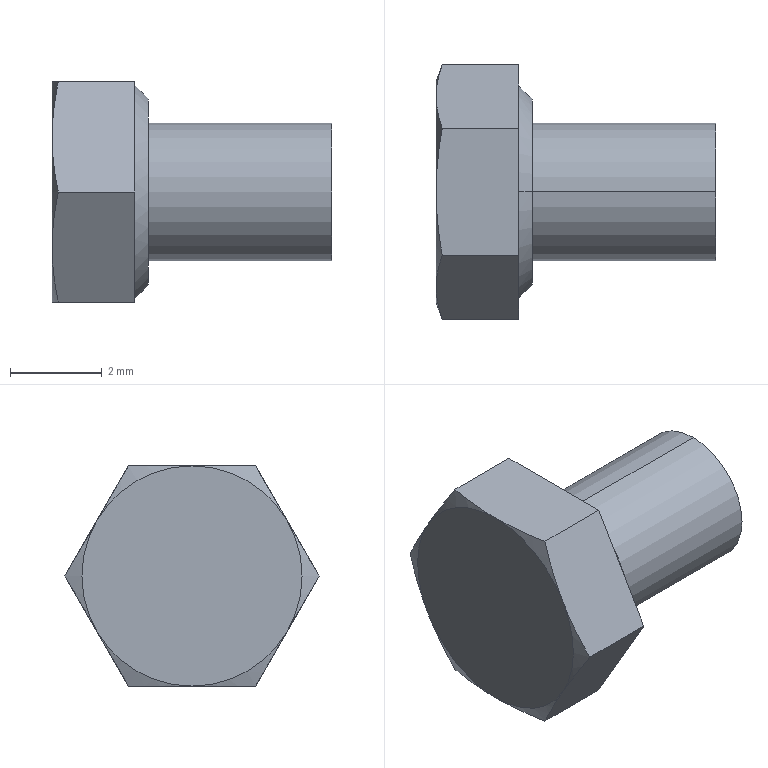Part | SolidWorks | features RevCut 3, Boss 1, Chamfer 1, Extrusion 1, Fillet 1, ICE 1, LPattern 1, Scale 1 | 1 solid | 20 faces | box 6.1 x 5.543 x 4.8 mm | volume 68.566 mm3 | plane 10 | cone 8 | cylinder 2 | commonest cylinder face diameters 3 x2
STEP:
#1=CARTESIAN_POINT('',(4.17,-0.000000444,2.022));
#2=VERTEX_POINT('',#1);
#3=CARTESIAN_POINT('',(4.17,-0.000000444,-2.022));
#4=VERTEX_POINT('',#3);
#5=CARTESIAN_POINT('',(4.17,-0.000000444,0.));
#6=DIRECTION('',(-1.,0.,0.));
#7=DIRECTION('',(0.,0.,1.));
#8=AXIS2_PLACEMENT_3D('',#5,#6,#7);
#9=CIRCLE('',#8,2.022);
#10=EDGE_CURVE('',#2,#4,#9,.T.);
#11=ORIENTED_EDGE('',*,*,#10,.T.);
#12=CARTESIAN_POINT('',(3.87,-0.000000444,-2.322));
#13=VERTEX_POINT('',#12);
#14=CARTESIAN_POINT('',(3.87,-0.000000444,-2.322));
#15=DIRECTION('',(-0.7071,0.,-0.7071));
#16=VECTOR('',#15,1000.);
#17=LINE('',#14,#16);
#18=EDGE_CURVE('',#4,#13,#17,.T.);
#19=ORIENTED_EDGE('',*,*,#18,.T.);
#20=CARTESIAN_POINT('',(3.87,-0.000000444,2.322));
#21=VERTEX_POINT('',#20);
#22=CARTESIAN_POINT('',(3.87,-0.000000444,0.));
#23=DIRECTION('',(-1.,0.,0.));
#24=DIRECTION('',(0.,0.,1.));
#25=AXIS2_PLACEMENT_3D('',#22,#23,#24);
#26=CIRCLE('',#25,2.322);
#27=EDGE_CURVE('',#21,#13,#26,.T.);
#28=ORIENTED_EDGE('',*,*,#27,.F.);
#29=CARTESIAN_POINT('',(3.87,-0.000000444,2.322));
#30=DIRECTION('',(-0.7071,0.,0.7071));
#31=VECTOR('',#30,1000.);
#32=LINE('',#29,#31);
#33=EDGE_CURVE('',#2,#21,#32,.T.);
#34=ORIENTED_EDGE('',*,*,#33,.F.);
#35=EDGE_LOOP('',(#11,#19,#28,#34));
#36=FACE_OUTER_BOUND('',#35,.T.);
#37=CARTESIAN_POINT('',(3.87,-0.000000444,0.));
#38=DIRECTION('',(-1.,0.,0.));
#39=DIRECTION('',(0.,0.,1.));
#40=AXIS2_PLACEMENT_3D('',#37,#38,#39);
#41=CONICAL_SURFACE('',#40,2.322,0.7854);
#42=ADVANCED_FACE('',(#36),#41,.T.);
#43=CARTESIAN_POINT('',(8.17,-0.000000444,-1.5));
#44=VERTEX_POINT('',#43);
#45=CARTESIAN_POINT('',(8.17,-0.000000444,1.5));
#46=VERTEX_POINT('',#45);
#47=CARTESIAN_POINT('',(8.17,-0.000000444,0.));
#48=DIRECTION('',(1.,0.,0.));
#49=DIRECTION('',(0.,0.,-1.));
#50=AXIS2_PLACEMENT_3D('',#47,#48,#49);
#51=CIRCLE('',#50,1.5);
#52=EDGE_CURVE('',#44,#46,#51,.T.);
#53=ORIENTED_EDGE('',*,*,#52,.F.);
#54=CARTESIAN_POINT('',(4.17,-0.000000444,-1.5));
#55=VERTEX_POINT('',#54);
#56=CARTESIAN_POINT('',(10.17,-0.000000444,-1.5));
#57=DIRECTION('',(-1.,0.,0.));
#58=VECTOR('',#57,1000.);
#59=LINE('',#56,#58);
#60=EDGE_CURVE('',#44,#55,#59,.T.);
#61=ORIENTED_EDGE('',*,*,#60,.T.);
#62=CARTESIAN_POINT('',(4.17,-0.000000444,1.5));
#63=VERTEX_POINT('',#62);
#64=CARTESIAN_POINT('',(4.17,-0.000000444,0.));
#65=DIRECTION('',(1.,0.,0.));
#66=DIRECTION('',(0.,0.,1.));
#67=AXIS2_PLACEMENT_3D('',#64,#65,#66);
#68=CIRCLE('',#67,1.5);
#69=EDGE_CURVE('',#55,#63,#68,.T.);
#70=ORIENTED_EDGE('',*,*,#69,.T.);
#71=CARTESIAN_POINT('',(10.17,-0.000000444,1.5));
#72=DIRECTION('',(-1.,0.,0.));
#73=VECTOR('',#72,1000.);
#74=LINE('',#71,#73);
#75=EDGE_CURVE('',#46,#63,#74,.T.);
#76=ORIENTED_EDGE('',*,*,#75,.F.);
#77=EDGE_LOOP('',(#53,#61,#70,#76));
#78=FACE_OUTER_BOUND('',#77,.T.);
#79=CARTESIAN_POINT('',(10.17,-0.000000444,0.));
#80=DIRECTION('',(-1.,0.,0.));
#81=DIRECTION('',(0.,0.,1.));
#82=AXIS2_PLACEMENT_3D('',#79,#80,#81);
#83=CYLINDRICAL_SURFACE('',#82,1.5);
#84=ADVANCED_FACE('',(#78),#83,.T.);
#85=ORIENTED_EDGE('',*,*,#60,.F.);
#86=CARTESIAN_POINT('',(8.17,-0.000000444,0.));
#87=DIRECTION('',(1.,0.,0.));
#88=DIRECTION('',(0.,0.,-1.));
#89=AXIS2_PLACEMENT_3D('',#86,#87,#88);
#90=CIRCLE('',#89,1.5);
#91=EDGE_CURVE('',#46,#44,#90,.T.);
#92=ORIENTED_EDGE('',*,*,#91,.F.);
#93=ORIENTED_EDGE('',*,*,#75,.T.);
#94=CARTESIAN_POINT('',(4.17,-0.000000444,0.));
#95=DIRECTION('',(1.,0.,0.));
#96=DIRECTION('',(0.,0.,1.));
#97=AXIS2_PLACEMENT_3D('',#94,#95,#96);
#98=CIRCLE('',#97,1.5);
#99=EDGE_CURVE('',#63,#55,#98,.T.);
#100=ORIENTED_EDGE('',*,*,#99,.T.);
#101=EDGE_LOOP('',(#85,#92,#93,#100));
#102=FACE_OUTER_BOUND('',#101,.T.);
#103=CARTESIAN_POINT('',(10.17,-0.000000444,0.));
#104=DIRECTION('',(-1.,0.,0.));
#105=DIRECTION('',(0.,0.,1.));
#106=AXIS2_PLACEMENT_3D('',#103,#104,#105);
#107=CYLINDRICAL_SURFACE('',#106,1.5);
#108=ADVANCED_FACE('',(#102),#107,.T.);
#109=ORIENTED_EDGE('',*,*,#10,.F.);
#110=CARTESIAN_POINT('',(4.17,-0.000000444,0.));
#111=DIRECTION('',(-1.,0.,0.));
#112=DIRECTION('',(0.,0.,1.));
#113=AXIS2_PLACEMENT_3D('',#110,#111,#112);
#114=CIRCLE('',#113,2.022);
#115=EDGE_CURVE('',#4,#2,#114,.T.);
#116=ORIENTED_EDGE('',*,*,#115,.F.);
#117=EDGE_LOOP('',(#109,#116));
#118=FACE_OUTER_BOUND('',#117,.T.);
#119=ORIENTED_EDGE('',*,*,#99,.F.);
#120=ORIENTED_EDGE('',*,*,#69,.F.);
#121=EDGE_LOOP('',(#119,#120));
#122=FACE_BOUND('',#121,.T.);
#123=CARTESIAN_POINT('',(4.17,-0.000000444,4.8));
#124=DIRECTION('',(-1.,0.,0.));
#125=DIRECTION('',(0.,0.,1.));
#126=AXIS2_PLACEMENT_3D('',#123,#124,#125);
#127=PLANE('',#126);
#128=ADVANCED_FACE('',(#118,#122),#127,.F.);
#129=CARTESIAN_POINT('',(2.205,-2.771,0.));
#130=VERTEX_POINT('',#129);
#131=CARTESIAN_POINT('',(2.07,-2.078,1.2));
#132=VERTEX_POINT('',#131);
#133=CARTESIAN_POINT('',(2.205,-2.771,0.));
#134=CARTESIAN_POINT('',(2.121,-2.54,0.4));
#135=CARTESIAN_POINT('',(2.07,-2.309,0.8));
#136=CARTESIAN_POINT('',(2.07,-2.078,1.2));
#137=B_SPLINE_CURVE_WITH_KNOTS('',3,(#133,#134,#135,#136),.UNSPECIFIED.,.F.,.F.,(4,4),(0.000000139,0.001386),.UNSPECIFIED.);
#138=EDGE_CURVE('',#130,#132,#137,.T.);
#139=ORIENTED_EDGE('',*,*,#138,.F.);
#140=CARTESIAN_POINT('',(3.87,-2.771,0.));
#141=VERTEX_POINT('',#140);
#142=CARTESIAN_POINT('',(4.17,-2.771,0.));
#143=DIRECTION('',(-1.,0.,0.));
#144=VECTOR('',#143,1000.);
#145=LINE('',#142,#144);
#146=EDGE_CURVE('',#141,#130,#145,.T.);
#147=ORIENTED_EDGE('',*,*,#146,.F.);
#148=CARTESIAN_POINT('',(3.87,-1.386,2.4));
#149=VERTEX_POINT('',#148);
#150=CARTESIAN_POINT('',(3.87,-1.386,2.4));
#151=DIRECTION('',(0.,-0.5,-0.866));
#152=VECTOR('',#151,1000.);
#153=LINE('',#150,#152);
#154=EDGE_CURVE('',#149,#141,#153,.T.);
#155=ORIENTED_EDGE('',*,*,#154,.F.);
#156=CARTESIAN_POINT('',(2.205,-1.386,2.4));
#157=VERTEX_POINT('',#156);
#158=CARTESIAN_POINT('',(4.17,-1.386,2.4));
#159=DIRECTION('',(-1.,0.,0.));
#160=VECTOR('',#159,1000.);
#161=LINE('',#158,#160);
#162=EDGE_CURVE('',#149,#157,#161,.T.);
#163=ORIENTED_EDGE('',*,*,#162,.T.);
#164=CARTESIAN_POINT('',(2.07,-2.078,1.2));
#165=CARTESIAN_POINT('',(2.07,-1.848,1.6));
#166=CARTESIAN_POINT('',(2.121,-1.617,2.));
#167=CARTESIAN_POINT('',(2.205,-1.386,2.4));
#168=B_SPLINE_CURVE_WITH_KNOTS('',3,(#164,#165,#166,#167),.UNSPECIFIED.,.F.,.F.,(4,4),(0.001386,0.002771),.UNSPECIFIED.);
#169=EDGE_CURVE('',#132,#157,#168,.T.);
#170=ORIENTED_EDGE('',*,*,#169,.F.);
#171=EDGE_LOOP('',(#139,#147,#155,#163,#170));
#172=FACE_OUTER_BOUND('',#171,.T.);
#173=CARTESIAN_POINT('',(4.17,-1.386,2.4));
#174=DIRECTION('',(0.,0.866,-0.5));
#175=DIRECTION('',(0.,0.5,0.866));
#176=AXIS2_PLACEMENT_3D('',#173,#174,#175);
#177=PLANE('',#176);
#178=ADVANCED_FACE('',(#172),#177,.F.);
#179=CARTESIAN_POINT('',(2.205,-1.386,-2.4));
#180=VERTEX_POINT('',#179);
#181=CARTESIAN_POINT('',(2.07,-2.078,-1.2));
#182=VERTEX_POINT('',#181);
#183=CARTESIAN_POINT('',(2.205,-1.386,-2.4));
#184=CARTESIAN_POINT('',(2.121,-1.617,-2.));
#185=CARTESIAN_POINT('',(2.07,-1.848,-1.6));
#186=CARTESIAN_POINT('',(2.07,-2.078,-1.2));
#187=B_SPLINE_CURVE_WITH_KNOTS('',3,(#183,#184,#185,#186),.UNSPECIFIED.,.F.,.F.,(4,4),(0.000000139,0.001386),.UNSPECIFIED.);
#188=EDGE_CURVE('',#180,#182,#187,.T.);
#189=ORIENTED_EDGE('',*,*,#188,.F.);
#190=CARTESIAN_POINT('',(3.87,-1.386,-2.4));
#191=VERTEX_POINT('',#190);
#192=CARTESIAN_POINT('',(4.17,-1.386,-2.4));
#193=DIRECTION('',(-1.,0.,0.));
#194=VECTOR('',#193,1000.);
#195=LINE('',#192,#194);
#196=EDGE_CURVE('',#191,#180,#195,.T.);
#197=ORIENTED_EDGE('',*,*,#196,.F.);
#198=CARTESIAN_POINT('',(3.87,-2.771,0.));
#199=DIRECTION('',(0.,0.5,-0.866));
#200=VECTOR('',#199,1000.);
#201=LINE('',#198,#200);
#202=EDGE_CURVE('',#141,#191,#201,.T.);
#203=ORIENTED_EDGE('',*,*,#202,.F.);
#204=ORIENTED_EDGE('',*,*,#146,.T.);
#205=CARTESIAN_POINT('',(2.07,-2.078,-1.2));
#206=CARTESIAN_POINT('',(2.07,-2.309,-0.8));
#207=CARTESIAN_POINT('',(2.121,-2.54,-0.4));
#208=CARTESIAN_POINT('',(2.205,-2.771,0.));
#209=B_SPLINE_CURVE_WITH_KNOTS('',3,(#205,#206,#207,#208),.UNSPECIFIED.,.F.,.F.,(4,4),(0.001386,0.002771),.UNSPECIFIED.);
#210=EDGE_CURVE('',#182,#130,#209,.T.);
#211=ORIENTED_EDGE('',*,*,#210,.F.);
#212=EDGE_LOOP('',(#189,#197,#203,#204,#211));
#213=FACE_OUTER_BOUND('',#212,.T.);
#214=CARTESIAN_POINT('',(4.17,-2.771,0.));
#215=DIRECTION('',(0.,0.866,0.5));
#216=DIRECTION('',(0.,-0.5,0.866));
#217=AXIS2_PLACEMENT_3D('',#214,#215,#216);
#218=PLANE('',#217);
#219=ADVANCED_FACE('',(#213),#218,.F.);
#220=CARTESIAN_POINT('',(2.205,1.386,-2.4));
#221=VERTEX_POINT('',#220);
#222=CARTESIAN_POINT('',(2.07,-0.000000444,-2.4));
#223=VERTEX_POINT('',#222);
#224=CARTESIAN_POINT('',(2.205,1.386,-2.4));
#225=CARTESIAN_POINT('',(2.121,0.925,-2.4));
#226=CARTESIAN_POINT('',(2.07,0.4628,-2.4));
#227=CARTESIAN_POINT('',(2.07,-0.000000444,-2.4));
#228=B_SPLINE_CURVE_WITH_KNOTS('',3,(#224,#225,#226,#227),.UNSPECIFIED.,.F.,.F.,(4,4),(0.004997,0.006394),.UNSPECIFIED.);
#229=EDGE_CURVE('',#221,#223,#228,.T.);
#230=ORIENTED_EDGE('',*,*,#229,.F.);
#231=CARTESIAN_POINT('',(3.87,1.386,-2.4));
#232=VERTEX_POINT('',#231);
#233=CARTESIAN_POINT('',(4.17,1.386,-2.4));
#234=DIRECTION('',(-1.,0.,0.));
#235=VECTOR('',#234,1000.);
#236=LINE('',#233,#235);
#237=EDGE_CURVE('',#232,#221,#236,.T.);
#238=ORIENTED_EDGE('',*,*,#237,.F.);
#239=CARTESIAN_POINT('',(3.87,-1.386,-2.4));
#240=DIRECTION('',(0.,1.,0.));
#241=VECTOR('',#240,1000.);
#242=LINE('',#239,#241);
#243=EDGE_CURVE('',#191,#232,#242,.T.);
#244=ORIENTED_EDGE('',*,*,#243,.F.);
#245=ORIENTED_EDGE('',*,*,#196,.T.);
#246=CARTESIAN_POINT('',(2.07,-0.000000444,-2.4));
#247=CARTESIAN_POINT('',(2.07,-0.4615,-2.4));
#248=CARTESIAN_POINT('',(2.121,-0.9268,-2.4));
#249=CARTESIAN_POINT('',(2.205,-1.386,-2.4));
#250=B_SPLINE_CURVE_WITH_KNOTS('',3,(#246,#247,#248,#249),.UNSPECIFIED.,.F.,.F.,(4,4),(0.006394,0.007787),.UNSPECIFIED.);
#251=EDGE_CURVE('',#223,#180,#250,.T.);
#252=ORIENTED_EDGE('',*,*,#251,.F.);
#253=EDGE_LOOP('',(#230,#238,#244,#245,#252));
#254=FACE_OUTER_BOUND('',#253,.T.);
#255=CARTESIAN_POINT('',(4.17,-1.386,-2.4));
#256=DIRECTION('',(0.,0.,1.));
#257=DIRECTION('',(0.,-1.,0.));
#258=AXIS2_PLACEMENT_3D('',#255,#256,#257);
#259=PLANE('',#258);
#260=ADVANCED_FACE('',(#254),#259,.F.);
#261=CARTESIAN_POINT('',(2.205,2.771,0.));
#262=VERTEX_POINT('',#261);
#263=CARTESIAN_POINT('',(2.07,2.078,-1.2));
#264=VERTEX_POINT('',#263);
#265=CARTESIAN_POINT('',(2.205,2.771,0.));
#266=CARTESIAN_POINT('',(2.121,2.54,-0.4));
#267=CARTESIAN_POINT('',(2.07,2.309,-0.8));
#268=CARTESIAN_POINT('',(2.07,2.078,-1.2));
#269=B_SPLINE_CURVE_WITH_KNOTS('',3,(#265,#266,#267,#268),.UNSPECIFIED.,.F.,.F.,(4,4),(0.000000139,0.001386),.UNSPECIFIED.);
#270=EDGE_CURVE('',#262,#264,#269,.T.);
#271=ORIENTED_EDGE('',*,*,#270,.F.);
#272=CARTESIAN_POINT('',(3.87,2.771,0.));
#273=VERTEX_POINT('',#272);
#274=CARTESIAN_POINT('',(4.17,2.771,0.));
#275=DIRECTION('',(-1.,0.,0.));
#276=VECTOR('',#275,1000.);
#277=LINE('',#274,#276);
#278=EDGE_CURVE('',#273,#262,#277,.T.);
#279=ORIENTED_EDGE('',*,*,#278,.F.);
#280=CARTESIAN_POINT('',(3.87,1.386,-2.4));
#281=DIRECTION('',(0.,0.5,0.866));
#282=VECTOR('',#281,1000.);
#283=LINE('',#280,#282);
#284=EDGE_CURVE('',#232,#273,#283,.T.);
#285=ORIENTED_EDGE('',*,*,#284,.F.);
#286=ORIENTED_EDGE('',*,*,#237,.T.);
#287=CARTESIAN_POINT('',(2.07,2.078,-1.2));
#288=CARTESIAN_POINT('',(2.07,1.848,-1.6));
#289=CARTESIAN_POINT('',(2.121,1.617,-2.));
#290=CARTESIAN_POINT('',(2.205,1.386,-2.4));
#291=B_SPLINE_CURVE_WITH_KNOTS('',3,(#287,#288,#289,#290),.UNSPECIFIED.,.F.,.F.,(4,4),(0.001386,0.002771),.UNSPECIFIED.);
#292=EDGE_CURVE('',#264,#221,#291,.T.);
#293=ORIENTED_EDGE('',*,*,#292,.F.);
#294=EDGE_LOOP('',(#271,#279,#285,#286,#293));
#295=FACE_OUTER_BOUND('',#294,.T.);
#296=CARTESIAN_POINT('',(4.17,1.386,-2.4));
#297=DIRECTION('',(0.,-0.866,0.5));
#298=DIRECTION('',(0.,-0.5,-0.866));
#299=AXIS2_PLACEMENT_3D('',#296,#297,#298);
#300=PLANE('',#299);
#301=ADVANCED_FACE('',(#295),#300,.F.);
#302=CARTESIAN_POINT('',(2.205,1.386,2.4));
#303=VERTEX_POINT('',#302);
#304=CARTESIAN_POINT('',(2.07,2.078,1.2));
#305=VERTEX_POINT('',#304);
#306=CARTESIAN_POINT('',(2.205,1.386,2.4));
#307=CARTESIAN_POINT('',(2.121,1.617,2.));
#308=CARTESIAN_POINT('',(2.07,1.848,1.6));
#309=CARTESIAN_POINT('',(2.07,2.078,1.2));
#310=B_SPLINE_CURVE_WITH_KNOTS('',3,(#306,#307,#308,#309),.UNSPECIFIED.,.F.,.F.,(4,4),(0.000000139,0.001386),.UNSPECIFIED.);
#311=EDGE_CURVE('',#303,#305,#310,.T.);
#312=ORIENTED_EDGE('',*,*,#311,.F.);
#313=CARTESIAN_POINT('',(3.87,1.386,2.4));
#314=VERTEX_POINT('',#313);
#315=CARTESIAN_POINT('',(4.17,1.386,2.4));
#316=DIRECTION('',(-1.,0.,0.));
#317=VECTOR('',#316,1000.);
#318=LINE('',#315,#317);
#319=EDGE_CURVE('',#314,#303,#318,.T.);
#320=ORIENTED_EDGE('',*,*,#319,.F.);
#321=CARTESIAN_POINT('',(3.87,2.771,0.));
#322=DIRECTION('',(0.,-0.5,0.866));
#323=VECTOR('',#322,1000.);
#324=LINE('',#321,#323);
#325=EDGE_CURVE('',#273,#314,#324,.T.);
#326=ORIENTED_EDGE('',*,*,#325,.F.);
#327=ORIENTED_EDGE('',*,*,#278,.T.);
#328=CARTESIAN_POINT('',(2.07,2.078,1.2));
#329=CARTESIAN_POINT('',(2.07,2.309,0.8));
#330=CARTESIAN_POINT('',(2.121,2.54,0.4));
#331=CARTESIAN_POINT('',(2.205,2.771,0.));
#332=B_SPLINE_CURVE_WITH_KNOTS('',3,(#328,#329,#330,#331),.UNSPECIFIED.,.F.,.F.,(4,4),(0.001386,0.002771),.UNSPECIFIED.);
#333=EDGE_CURVE('',#305,#262,#332,.T.);
#334=ORIENTED_EDGE('',*,*,#333,.F.);
#335=EDGE_LOOP('',(#312,#320,#326,#327,#334));
#336=FACE_OUTER_BOUND('',#335,.T.);
#337=CARTESIAN_POINT('',(4.17,2.771,0.));
#338=DIRECTION('',(0.,-0.866,-0.5));
#339=DIRECTION('',(0.,0.5,-0.866));
#340=AXIS2_PLACEMENT_3D('',#337,#338,#339);
#341=PLANE('',#340);
#342=ADVANCED_FACE('',(#336),#341,.F.);
#343=CARTESIAN_POINT('',(2.07,-0.000000444,2.4));
#344=VERTEX_POINT('',#343);
#345=CARTESIAN_POINT('',(2.205,-1.386,2.4));
#346=CARTESIAN_POINT('',(2.121,-0.9268,2.4));
#347=CARTESIAN_POINT('',(2.07,-0.4615,2.4));
#348=CARTESIAN_POINT('',(2.07,-0.000000444,2.4));
#349=B_SPLINE_CURVE_WITH_KNOTS('',3,(#345,#346,#347,#348),.UNSPECIFIED.,.F.,.F.,(4,4),(0.002357,0.003754),.UNSPECIFIED.);
#350=EDGE_CURVE('',#157,#344,#349,.T.);
#351=ORIENTED_EDGE('',*,*,#350,.F.);
#352=ORIENTED_EDGE('',*,*,#162,.F.);
#353=CARTESIAN_POINT('',(3.87,1.386,2.4));
#354=DIRECTION('',(0.,-1.,0.));
#355=VECTOR('',#354,1000.);
#356=LINE('',#353,#355);
#357=EDGE_CURVE('',#314,#149,#356,.T.);
#358=ORIENTED_EDGE('',*,*,#357,.F.);
#359=ORIENTED_EDGE('',*,*,#319,.T.);
#360=CARTESIAN_POINT('',(2.07,-0.000000444,2.4));
#361=CARTESIAN_POINT('',(2.07,0.4628,2.4));
#362=CARTESIAN_POINT('',(2.121,0.925,2.4));
#363=CARTESIAN_POINT('',(2.205,1.386,2.4));
#364=B_SPLINE_CURVE_WITH_KNOTS('',3,(#360,#361,#362,#363),.UNSPECIFIED.,.F.,.F.,(4,4),(0.003754,0.005154),.UNSPECIFIED.);
#365=EDGE_CURVE('',#344,#303,#364,.T.);
#366=ORIENTED_EDGE('',*,*,#365,.F.);
#367=EDGE_LOOP('',(#351,#352,#358,#359,#366));
#368=FACE_OUTER_BOUND('',#367,.T.);
#369=CARTESIAN_POINT('',(4.17,1.386,2.4));
#370=DIRECTION('',(0.,0.,-1.));
#371=DIRECTION('',(-1.,0.,0.));
#372=AXIS2_PLACEMENT_3D('',#369,#370,#371);
#373=PLANE('',#372);
#374=ADVANCED_FACE('',(#368),#373,.F.);
#375=ORIENTED_EDGE('',*,*,#27,.T.);
#376=CARTESIAN_POINT('',(3.87,-0.000000444,0.));
#377=DIRECTION('',(-1.,0.,0.));
#378=DIRECTION('',(0.,0.,1.));
#379=AXIS2_PLACEMENT_3D('',#376,#377,#378);
#380=CIRCLE('',#379,2.322);
#381=EDGE_CURVE('',#13,#21,#380,.T.);
#382=ORIENTED_EDGE('',*,*,#381,.T.);
#383=EDGE_LOOP('',(#375,#382));
#384=FACE_BOUND('',#383,.T.);
#385=ORIENTED_EDGE('',*,*,#154,.T.);
#386=ORIENTED_EDGE('',*,*,#202,.T.);
#387=ORIENTED_EDGE('',*,*,#243,.T.);
#388=ORIENTED_EDGE('',*,*,#284,.T.);
#389=ORIENTED_EDGE('',*,*,#325,.T.);
#390=ORIENTED_EDGE('',*,*,#357,.T.);
#391=EDGE_LOOP('',(#385,#386,#387,#388,#389,#390));
#392=FACE_OUTER_BOUND('',#391,.T.);
#393=CARTESIAN_POINT('',(3.87,2.322,0.));
#394=DIRECTION('',(1.,0.,0.));
#395=DIRECTION('',(0.,0.,-1.));
#396=AXIS2_PLACEMENT_3D('',#393,#394,#395);
#397=PLANE('',#396);
#398=ADVANCED_FACE('',(#384,#392),#397,.T.);
#399=ORIENTED_EDGE('',*,*,#18,.F.);
#400=ORIENTED_EDGE('',*,*,#115,.T.);
#401=ORIENTED_EDGE('',*,*,#33,.T.);
#402=ORIENTED_EDGE('',*,*,#381,.F.);
#403=EDGE_LOOP('',(#399,#400,#401,#402));
#404=FACE_OUTER_BOUND('',#403,.T.);
#405=CARTESIAN_POINT('',(3.87,-0.000000444,0.));
#406=DIRECTION('',(-1.,0.,0.));
#407=DIRECTION('',(0.,0.,1.));
#408=AXIS2_PLACEMENT_3D('',#405,#406,#407);
#409=CONICAL_SURFACE('',#408,2.322,0.7854);
#410=ADVANCED_FACE('',(#404),#409,.T.);
#411=ORIENTED_EDGE('',*,*,#169,.T.);
#412=ORIENTED_EDGE('',*,*,#350,.T.);
#413=CARTESIAN_POINT('',(2.07,-0.000000444,0.));
#414=DIRECTION('',(-1.,0.,0.));
#415=DIRECTION('',(0.,0.,1.));
#416=AXIS2_PLACEMENT_3D('',#413,#414,#415);
#417=CIRCLE('',#416,2.4);
#418=EDGE_CURVE('',#132,#344,#417,.T.);
#419=ORIENTED_EDGE('',*,*,#418,.F.);
#420=EDGE_LOOP('',(#411,#412,#419));
#421=FACE_OUTER_BOUND('',#420,.T.);
#422=CARTESIAN_POINT('',(2.07,-0.000000444,0.));
#423=DIRECTION('',(1.,0.,0.));
#424=DIRECTION('',(0.,0.,-1.));
#425=AXIS2_PLACEMENT_3D('',#422,#423,#424);
#426=CONICAL_SURFACE('',#425,2.4,1.222);
#427=ADVANCED_FACE('',(#421),#426,.T.);
#428=ORIENTED_EDGE('',*,*,#210,.T.);
#429=ORIENTED_EDGE('',*,*,#138,.T.);
#430=CARTESIAN_POINT('',(2.07,-0.000000444,0.));
#431=DIRECTION('',(-1.,0.,0.));
#432=DIRECTION('',(0.,0.,1.));
#433=AXIS2_PLACEMENT_3D('',#430,#431,#432);
#434=CIRCLE('',#433,2.4);
#435=EDGE_CURVE('',#182,#132,#434,.T.);
#436=ORIENTED_EDGE('',*,*,#435,.F.);
#437=EDGE_LOOP('',(#428,#429,#436));
#438=FACE_OUTER_BOUND('',#437,.T.);
#439=CARTESIAN_POINT('',(2.07,-0.000000444,0.));
#440=DIRECTION('',(1.,0.,0.));
#441=DIRECTION('',(0.,0.,-1.));
#442=AXIS2_PLACEMENT_3D('',#439,#440,#441);
#443=CONICAL_SURFACE('',#442,2.4,1.222);
#444=ADVANCED_FACE('',(#438),#443,.T.);
#445=ORIENTED_EDGE('',*,*,#251,.T.);
#446=ORIENTED_EDGE('',*,*,#188,.T.);
#447=CARTESIAN_POINT('',(2.07,-0.000000444,0.));
#448=DIRECTION('',(-1.,0.,0.));
#449=DIRECTION('',(0.,0.,1.));
#450=AXIS2_PLACEMENT_3D('',#447,#448,#449);
#451=CIRCLE('',#450,2.4);
#452=EDGE_CURVE('',#223,#182,#451,.T.);
#453=ORIENTED_EDGE('',*,*,#452,.F.);
#454=EDGE_LOOP('',(#445,#446,#453));
#455=FACE_OUTER_BOUND('',#454,.T.);
#456=CARTESIAN_POINT('',(2.07,-0.000000444,0.));
#457=DIRECTION('',(1.,0.,0.));
#458=DIRECTION('',(0.,0.,-1.));
#459=AXIS2_PLACEMENT_3D('',#456,#457,#458);
#460=CONICAL_SURFACE('',#459,2.4,1.222);
#461=ADVANCED_FACE('',(#455),#460,.T.);
#462=ORIENTED_EDGE('',*,*,#229,.T.);
#463=CARTESIAN_POINT('',(2.07,-0.000000444,0.));
#464=DIRECTION('',(-1.,0.,0.));
#465=DIRECTION('',(0.,0.,1.));
#466=AXIS2_PLACEMENT_3D('',#463,#464,#465);
#467=CIRCLE('',#466,2.4);
#468=EDGE_CURVE('',#264,#223,#467,.T.);
#469=ORIENTED_EDGE('',*,*,#468,.F.);
#470=ORIENTED_EDGE('',*,*,#292,.T.);
#471=EDGE_LOOP('',(#462,#469,#470));
#472=FACE_OUTER_BOUND('',#471,.T.);
#473=CARTESIAN_POINT('',(2.07,-0.000000444,0.));
#474=DIRECTION('',(1.,0.,0.));
#475=DIRECTION('',(0.,0.,-1.));
#476=AXIS2_PLACEMENT_3D('',#473,#474,#475);
#477=CONICAL_SURFACE('',#476,2.4,1.222);
#478=ADVANCED_FACE('',(#472),#477,.T.);
#479=ORIENTED_EDGE('',*,*,#270,.T.);
#480=CARTESIAN_POINT('',(2.07,-0.000000444,0.));
#481=DIRECTION('',(-1.,0.,0.));
#482=DIRECTION('',(0.,0.,1.));
#483=AXIS2_PLACEMENT_3D('',#480,#481,#482);
#484=CIRCLE('',#483,2.4);
#485=EDGE_CURVE('',#305,#264,#484,.T.);
#486=ORIENTED_EDGE('',*,*,#485,.F.);
#487=ORIENTED_EDGE('',*,*,#333,.T.);
#488=EDGE_LOOP('',(#479,#486,#487));
#489=FACE_OUTER_BOUND('',#488,.T.);
#490=CARTESIAN_POINT('',(2.07,-0.000000444,0.));
#491=DIRECTION('',(1.,0.,0.));
#492=DIRECTION('',(0.,0.,-1.));
#493=AXIS2_PLACEMENT_3D('',#490,#491,#492);
#494=CONICAL_SURFACE('',#493,2.4,1.222);
#495=ADVANCED_FACE('',(#489),#494,.T.);
#496=ORIENTED_EDGE('',*,*,#311,.T.);
#497=CARTESIAN_POINT('',(2.07,-0.000000444,0.));
#498=DIRECTION('',(-1.,0.,0.));
#499=DIRECTION('',(0.,0.,1.));
#500=AXIS2_PLACEMENT_3D('',#497,#498,#499);
#501=CIRCLE('',#500,2.4);
#502=EDGE_CURVE('',#344,#305,#501,.T.);
#503=ORIENTED_EDGE('',*,*,#502,.F.);
#504=ORIENTED_EDGE('',*,*,#365,.T.);
#505=EDGE_LOOP('',(#496,#503,#504));
#506=FACE_OUTER_BOUND('',#505,.T.);
#507=CARTESIAN_POINT('',(2.07,-0.000000444,0.));
#508=DIRECTION('',(1.,0.,0.));
#509=DIRECTION('',(0.,0.,-1.));
#510=AXIS2_PLACEMENT_3D('',#507,#508,#509);
#511=CONICAL_SURFACE('',#510,2.4,1.222);
#512=ADVANCED_FACE('',(#506),#511,.T.);
#513=ORIENTED_EDGE('',*,*,#418,.T.);
#514=ORIENTED_EDGE('',*,*,#502,.T.);
#515=ORIENTED_EDGE('',*,*,#485,.T.);
#516=ORIENTED_EDGE('',*,*,#468,.T.);
#517=ORIENTED_EDGE('',*,*,#452,.T.);
#518=ORIENTED_EDGE('',*,*,#435,.T.);
#519=EDGE_LOOP('',(#513,#514,#515,#516,#517,#518));
#520=FACE_OUTER_BOUND('',#519,.T.);
#521=CARTESIAN_POINT('',(2.07,-0.000000444,4.8));
#522=DIRECTION('',(-1.,0.,0.));
#523=DIRECTION('',(0.,0.,1.));
#524=AXIS2_PLACEMENT_3D('',#521,#522,#523);
#525=PLANE('',#524);
#526=ADVANCED_FACE('',(#520),#525,.T.);
#527=ORIENTED_EDGE('',*,*,#91,.T.);
#528=ORIENTED_EDGE('',*,*,#52,.T.);
#529=EDGE_LOOP('',(#527,#528));
#530=FACE_OUTER_BOUND('',#529,.T.);
#531=CARTESIAN_POINT('',(8.17,0.,0.));
#532=DIRECTION('',(1.,0.,0.));
#533=DIRECTION('',(0.,0.,-1.));
#534=AXIS2_PLACEMENT_3D('',#531,#532,#533);
#535=PLANE('',#534);
#536=ADVANCED_FACE('',(#530),#535,.T.);
#537=CLOSED_SHELL('',(#42,#84,#108,#128,#178,#219,#260,#301,#342,#374,#398,#410,#427,#444,#461,#478,#495,#512,#526,#536));
#538=MANIFOLD_SOLID_BREP('',#537);
#539=CARTESIAN_POINT('',(0.,0.,0.));
#540=DIRECTION('',(0.,0.,1.));
#541=DIRECTION('',(1.,0.,0.));
#542=AXIS2_PLACEMENT_3D('',#539,#540,#541);
#543=(LENGTH_UNIT()NAMED_UNIT(*)SI_UNIT(.MILLI.,.METRE.));
#544=UNCERTAINTY_MEASURE_WITH_UNIT(LENGTH_MEASURE(0.00001),#543,'','');
#545=(NAMED_UNIT(*)PLANE_ANGLE_UNIT()SI_UNIT($,.RADIAN.));
#546=(NAMED_UNIT(*)SI_UNIT($,.STERADIAN.)SOLID_ANGLE_UNIT());
#547=(GEOMETRIC_REPRESENTATION_CONTEXT(3)GLOBAL_UNCERTAINTY_ASSIGNED_CONTEXT((#544))GLOBAL_UNIT_ASSIGNED_CONTEXT((#543,#545,#546))REPRESENTATION_CONTEXT('',''));
#548=ADVANCED_BREP_SHAPE_REPRESENTATION('',(#538,#542),#547);